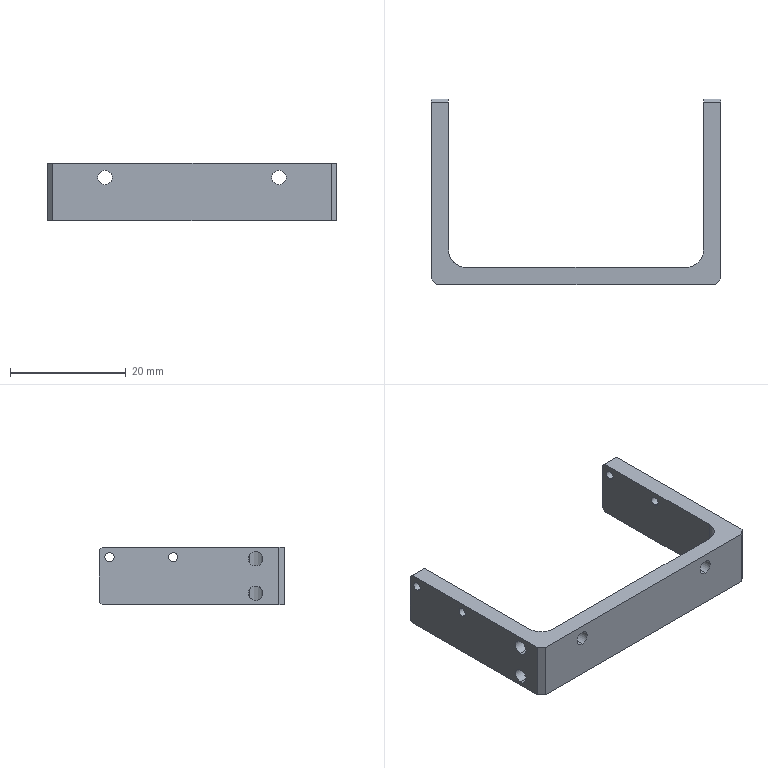Part | SolidWorks | features HoleWzd 3, Chamfer 2, Extrusion 1, Fillet 1, ICE 1 | 1 solid | 34 faces | box 50 x 32 x 10 mm | volume 3182 mm3 | cylinder 18 | plane 16 | commonest cylinder face diameters 1.6 x8 2.5 x8 6 x2
STEP:
#1=CARTESIAN_POINT('',(-21.828,-11.,-4.25));
#2=VERTEX_POINT('',#1);
#3=CARTESIAN_POINT('',(-21.828,-11.,-1.75));
#4=VERTEX_POINT('',#3);
#5=CARTESIAN_POINT('',(-21.828,-11.,-4.25));
#6=CARTESIAN_POINT('',(-21.768,-11.17,-4.25));
#7=CARTESIAN_POINT('',(-21.693,-11.333,-4.215));
#8=CARTESIAN_POINT('',(-21.526,-11.627,-4.093));
#9=CARTESIAN_POINT('',(-21.434,-11.759,-4.005));
#10=CARTESIAN_POINT('',(-21.301,-11.926,-3.843));
#11=CARTESIAN_POINT('',(-21.257,-11.977,-3.784));
#12=CARTESIAN_POINT('',(-21.174,-12.068,-3.654));
#13=CARTESIAN_POINT('',(-21.134,-12.109,-3.583));
#14=CARTESIAN_POINT('',(-21.031,-12.21,-3.356));
#15=CARTESIAN_POINT('',(-20.984,-12.25,-3.178));
#16=CARTESIAN_POINT('',(-20.985,-12.25,-2.817));
#17=CARTESIAN_POINT('',(-21.032,-12.209,-2.642));
#18=CARTESIAN_POINT('',(-21.17,-12.073,-2.338));
#19=CARTESIAN_POINT('',(-21.258,-11.981,-2.209));
#20=CARTESIAN_POINT('',(-21.437,-11.755,-1.992));
#21=CARTESIAN_POINT('',(-21.527,-11.625,-1.906));
#22=CARTESIAN_POINT('',(-21.695,-11.329,-1.784));
#23=CARTESIAN_POINT('',(-21.768,-11.171,-1.75));
#24=CARTESIAN_POINT('',(-21.828,-11.,-1.75));
#25=B_SPLINE_CURVE_WITH_KNOTS('',3,(#5,#6,#7,#8,#9,#10,#11,#12,#13,#14,#15,#16,#17,#18,#19,#20,#21,#22,#23,#24),.UNSPECIFIED.,.F.,.F.,(4,2,2,2,2,2,2,2,2,4),(0.001173,0.001709,0.002246,0.002514,0.002782,0.003319,0.003855,0.004392,0.004928,0.005465),.UNSPECIFIED.);
#26=EDGE_CURVE('',#2,#4,#25,.T.);
#27=ORIENTED_EDGE('',*,*,#26,.F.);
#28=CARTESIAN_POINT('',(-25.,-11.,-4.25));
#29=VERTEX_POINT('',#28);
#30=CARTESIAN_POINT('',(-25.,-11.,-4.25));
#31=DIRECTION('',(-1.,0.,0.));
#32=VECTOR('',#31,1000.);
#33=LINE('',#30,#32);
#34=EDGE_CURVE('',#2,#29,#33,.T.);
#35=ORIENTED_EDGE('',*,*,#34,.T.);
#36=CARTESIAN_POINT('',(-25.,-11.,-1.75));
#37=VERTEX_POINT('',#36);
#38=CARTESIAN_POINT('',(-25.,-11.,-3.));
#39=DIRECTION('',(-1.,0.,0.));
#40=DIRECTION('',(0.,0.,1.));
#41=AXIS2_PLACEMENT_3D('',#38,#39,#40);
#42=CIRCLE('',#41,1.25);
#43=EDGE_CURVE('',#29,#37,#42,.T.);
#44=ORIENTED_EDGE('',*,*,#43,.T.);
#45=CARTESIAN_POINT('',(-25.,-11.,-1.75));
#46=DIRECTION('',(-1.,0.,0.));
#47=VECTOR('',#46,1000.);
#48=LINE('',#45,#47);
#49=EDGE_CURVE('',#4,#37,#48,.T.);
#50=ORIENTED_EDGE('',*,*,#49,.F.);
#51=EDGE_LOOP('',(#27,#35,#44,#50));
#52=FACE_OUTER_BOUND('',#51,.T.);
#53=CARTESIAN_POINT('',(-25.,-11.,-3.));
#54=DIRECTION('',(-1.,0.,0.));
#55=DIRECTION('',(0.,0.,1.));
#56=AXIS2_PLACEMENT_3D('',#53,#54,#55);
#57=CYLINDRICAL_SURFACE('',#56,1.25);
#58=ADVANCED_FACE('',(#52),#57,.F.);
#59=CARTESIAN_POINT('',(-21.828,-11.,1.75));
#60=VERTEX_POINT('',#59);
#61=CARTESIAN_POINT('',(-21.828,-11.,4.25));
#62=VERTEX_POINT('',#61);
#63=CARTESIAN_POINT('',(-21.828,-11.,1.75));
#64=CARTESIAN_POINT('',(-21.768,-11.17,1.75));
#65=CARTESIAN_POINT('',(-21.693,-11.333,1.785));
#66=CARTESIAN_POINT('',(-21.526,-11.627,1.907));
#67=CARTESIAN_POINT('',(-21.434,-11.759,1.995));
#68=CARTESIAN_POINT('',(-21.301,-11.926,2.157));
#69=CARTESIAN_POINT('',(-21.257,-11.977,2.216));
#70=CARTESIAN_POINT('',(-21.174,-12.068,2.346));
#71=CARTESIAN_POINT('',(-21.134,-12.109,2.417));
#72=CARTESIAN_POINT('',(-21.031,-12.21,2.644));
#73=CARTESIAN_POINT('',(-20.984,-12.25,2.822));
#74=CARTESIAN_POINT('',(-20.985,-12.25,3.183));
#75=CARTESIAN_POINT('',(-21.032,-12.209,3.358));
#76=CARTESIAN_POINT('',(-21.17,-12.073,3.662));
#77=CARTESIAN_POINT('',(-21.258,-11.981,3.791));
#78=CARTESIAN_POINT('',(-21.437,-11.755,4.008));
#79=CARTESIAN_POINT('',(-21.527,-11.625,4.094));
#80=CARTESIAN_POINT('',(-21.695,-11.329,4.216));
#81=CARTESIAN_POINT('',(-21.768,-11.171,4.25));
#82=CARTESIAN_POINT('',(-21.828,-11.,4.25));
#83=B_SPLINE_CURVE_WITH_KNOTS('',3,(#63,#64,#65,#66,#67,#68,#69,#70,#71,#72,#73,#74,#75,#76,#77,#78,#79,#80,#81,#82),.UNSPECIFIED.,.F.,.F.,(4,2,2,2,2,2,2,2,2,4),(0.001173,0.001709,0.002246,0.002514,0.002782,0.003319,0.003855,0.004392,0.004928,0.005465),.UNSPECIFIED.);
#84=EDGE_CURVE('',#60,#62,#83,.T.);
#85=ORIENTED_EDGE('',*,*,#84,.F.);
#86=CARTESIAN_POINT('',(-25.,-11.,1.75));
#87=VERTEX_POINT('',#86);
#88=CARTESIAN_POINT('',(-25.,-11.,1.75));
#89=DIRECTION('',(-1.,0.,0.));
#90=VECTOR('',#89,1000.);
#91=LINE('',#88,#90);
#92=EDGE_CURVE('',#60,#87,#91,.T.);
#93=ORIENTED_EDGE('',*,*,#92,.T.);
#94=CARTESIAN_POINT('',(-25.,-11.,4.25));
#95=VERTEX_POINT('',#94);
#96=CARTESIAN_POINT('',(-25.,-11.,3.));
#97=DIRECTION('',(-1.,0.,0.));
#98=DIRECTION('',(0.,0.,1.));
#99=AXIS2_PLACEMENT_3D('',#96,#97,#98);
#100=CIRCLE('',#99,1.25);
#101=EDGE_CURVE('',#87,#95,#100,.T.);
#102=ORIENTED_EDGE('',*,*,#101,.T.);
#103=CARTESIAN_POINT('',(-25.,-11.,4.25));
#104=DIRECTION('',(-1.,0.,0.));
#105=VECTOR('',#104,1000.);
#106=LINE('',#103,#105);
#107=EDGE_CURVE('',#62,#95,#106,.T.);
#108=ORIENTED_EDGE('',*,*,#107,.F.);
#109=EDGE_LOOP('',(#85,#93,#102,#108));
#110=FACE_OUTER_BOUND('',#109,.T.);
#111=CARTESIAN_POINT('',(-25.,-11.,3.));
#112=DIRECTION('',(-1.,0.,0.));
#113=DIRECTION('',(0.,0.,1.));
#114=AXIS2_PLACEMENT_3D('',#111,#112,#113);
#115=CYLINDRICAL_SURFACE('',#114,1.25);
#116=ADVANCED_FACE('',(#110),#115,.F.);
#117=CARTESIAN_POINT('',(-15.,-13.,3.75));
#118=VERTEX_POINT('',#117);
#119=CARTESIAN_POINT('',(-15.,-13.,1.25));
#120=VERTEX_POINT('',#119);
#121=CARTESIAN_POINT('',(-15.,-13.,2.5));
#122=DIRECTION('',(0.,-1.,0.));
#123=DIRECTION('',(0.,0.,-1.));
#124=AXIS2_PLACEMENT_3D('',#121,#122,#123);
#125=CIRCLE('',#124,1.25);
#126=EDGE_CURVE('',#118,#120,#125,.T.);
#127=ORIENTED_EDGE('',*,*,#126,.F.);
#128=CARTESIAN_POINT('',(-15.,-16.,3.75));
#129=VERTEX_POINT('',#128);
#130=CARTESIAN_POINT('',(-15.,-16.,3.75));
#131=DIRECTION('',(0.,-1.,0.));
#132=VECTOR('',#131,1000.);
#133=LINE('',#130,#132);
#134=EDGE_CURVE('',#118,#129,#133,.T.);
#135=ORIENTED_EDGE('',*,*,#134,.T.);
#136=CARTESIAN_POINT('',(-15.,-16.,1.25));
#137=VERTEX_POINT('',#136);
#138=CARTESIAN_POINT('',(-15.,-16.,2.5));
#139=DIRECTION('',(0.,-1.,0.));
#140=DIRECTION('',(0.,0.,-1.));
#141=AXIS2_PLACEMENT_3D('',#138,#139,#140);
#142=CIRCLE('',#141,1.25);
#143=EDGE_CURVE('',#129,#137,#142,.T.);
#144=ORIENTED_EDGE('',*,*,#143,.T.);
#145=CARTESIAN_POINT('',(-15.,-16.,1.25));
#146=DIRECTION('',(0.,-1.,0.));
#147=VECTOR('',#146,1000.);
#148=LINE('',#145,#147);
#149=EDGE_CURVE('',#120,#137,#148,.T.);
#150=ORIENTED_EDGE('',*,*,#149,.F.);
#151=EDGE_LOOP('',(#127,#135,#144,#150));
#152=FACE_OUTER_BOUND('',#151,.T.);
#153=CARTESIAN_POINT('',(-15.,-16.,2.5));
#154=DIRECTION('',(0.,-1.,0.));
#155=DIRECTION('',(0.,0.,-1.));
#156=AXIS2_PLACEMENT_3D('',#153,#154,#155);
#157=CYLINDRICAL_SURFACE('',#156,1.25);
#158=ADVANCED_FACE('',(#152),#157,.F.);
#159=CARTESIAN_POINT('',(15.,-13.,3.75));
#160=VERTEX_POINT('',#159);
#161=CARTESIAN_POINT('',(15.,-13.,1.25));
#162=VERTEX_POINT('',#161);
#163=CARTESIAN_POINT('',(15.,-13.,2.5));
#164=DIRECTION('',(0.,-1.,0.));
#165=DIRECTION('',(0.,0.,-1.));
#166=AXIS2_PLACEMENT_3D('',#163,#164,#165);
#167=CIRCLE('',#166,1.25);
#168=EDGE_CURVE('',#160,#162,#167,.T.);
#169=ORIENTED_EDGE('',*,*,#168,.F.);
#170=CARTESIAN_POINT('',(15.,-16.,3.75));
#171=VERTEX_POINT('',#170);
#172=CARTESIAN_POINT('',(15.,-16.,3.75));
#173=DIRECTION('',(0.,-1.,0.));
#174=VECTOR('',#173,1000.);
#175=LINE('',#172,#174);
#176=EDGE_CURVE('',#160,#171,#175,.T.);
#177=ORIENTED_EDGE('',*,*,#176,.T.);
#178=CARTESIAN_POINT('',(15.,-16.,1.25));
#179=VERTEX_POINT('',#178);
#180=CARTESIAN_POINT('',(15.,-16.,2.5));
#181=DIRECTION('',(0.,-1.,0.));
#182=DIRECTION('',(0.,0.,-1.));
#183=AXIS2_PLACEMENT_3D('',#180,#181,#182);
#184=CIRCLE('',#183,1.25);
#185=EDGE_CURVE('',#171,#179,#184,.T.);
#186=ORIENTED_EDGE('',*,*,#185,.T.);
#187=CARTESIAN_POINT('',(15.,-16.,1.25));
#188=DIRECTION('',(0.,-1.,0.));
#189=VECTOR('',#188,1000.);
#190=LINE('',#187,#189);
#191=EDGE_CURVE('',#162,#179,#190,.T.);
#192=ORIENTED_EDGE('',*,*,#191,.F.);
#193=EDGE_LOOP('',(#169,#177,#186,#192));
#194=FACE_OUTER_BOUND('',#193,.T.);
#195=CARTESIAN_POINT('',(15.,-16.,2.5));
#196=DIRECTION('',(0.,-1.,0.));
#197=DIRECTION('',(0.,0.,-1.));
#198=AXIS2_PLACEMENT_3D('',#195,#196,#197);
#199=CYLINDRICAL_SURFACE('',#198,1.25);
#200=ADVANCED_FACE('',(#194),#199,.F.);
#201=CARTESIAN_POINT('',(22.,14.25,4.05));
#202=VERTEX_POINT('',#201);
#203=CARTESIAN_POINT('',(22.,14.25,2.45));
#204=VERTEX_POINT('',#203);
#205=CARTESIAN_POINT('',(22.,14.25,3.25));
#206=DIRECTION('',(1.,0.,0.));
#207=DIRECTION('',(0.,0.,-1.));
#208=AXIS2_PLACEMENT_3D('',#205,#206,#207);
#209=CIRCLE('',#208,0.8);
#210=EDGE_CURVE('',#202,#204,#209,.T.);
#211=ORIENTED_EDGE('',*,*,#210,.F.);
#212=CARTESIAN_POINT('',(25.,14.25,4.05));
#213=VERTEX_POINT('',#212);
#214=CARTESIAN_POINT('',(25.,14.25,4.05));
#215=DIRECTION('',(1.,0.,0.));
#216=VECTOR('',#215,1000.);
#217=LINE('',#214,#216);
#218=EDGE_CURVE('',#202,#213,#217,.T.);
#219=ORIENTED_EDGE('',*,*,#218,.T.);
#220=CARTESIAN_POINT('',(25.,14.25,2.45));
#221=VERTEX_POINT('',#220);
#222=CARTESIAN_POINT('',(25.,14.25,3.25));
#223=DIRECTION('',(1.,0.,0.));
#224=DIRECTION('',(0.,0.,-1.));
#225=AXIS2_PLACEMENT_3D('',#222,#223,#224);
#226=CIRCLE('',#225,0.8);
#227=EDGE_CURVE('',#213,#221,#226,.T.);
#228=ORIENTED_EDGE('',*,*,#227,.T.);
#229=CARTESIAN_POINT('',(25.,14.25,2.45));
#230=DIRECTION('',(1.,0.,0.));
#231=VECTOR('',#230,1000.);
#232=LINE('',#229,#231);
#233=EDGE_CURVE('',#204,#221,#232,.T.);
#234=ORIENTED_EDGE('',*,*,#233,.F.);
#235=EDGE_LOOP('',(#211,#219,#228,#234));
#236=FACE_OUTER_BOUND('',#235,.T.);
#237=CARTESIAN_POINT('',(25.,14.25,3.25));
#238=DIRECTION('',(1.,0.,0.));
#239=DIRECTION('',(0.,0.,-1.));
#240=AXIS2_PLACEMENT_3D('',#237,#238,#239);
#241=CYLINDRICAL_SURFACE('',#240,0.8);
#242=ADVANCED_FACE('',(#236),#241,.F.);
#243=CARTESIAN_POINT('',(-25.,14.25,4.05));
#244=VERTEX_POINT('',#243);
#245=CARTESIAN_POINT('',(-25.,14.25,2.45));
#246=VERTEX_POINT('',#245);
#247=CARTESIAN_POINT('',(-25.,14.25,3.25));
#248=DIRECTION('',(1.,0.,0.));
#249=DIRECTION('',(0.,0.,-1.));
#250=AXIS2_PLACEMENT_3D('',#247,#248,#249);
#251=CIRCLE('',#250,0.8);
#252=EDGE_CURVE('',#244,#246,#251,.T.);
#253=ORIENTED_EDGE('',*,*,#252,.F.);
#254=CARTESIAN_POINT('',(-22.,14.25,4.05));
#255=VERTEX_POINT('',#254);
#256=CARTESIAN_POINT('',(25.,14.25,4.05));
#257=DIRECTION('',(1.,0.,0.));
#258=VECTOR('',#257,1000.);
#259=LINE('',#256,#258);
#260=EDGE_CURVE('',#244,#255,#259,.T.);
#261=ORIENTED_EDGE('',*,*,#260,.T.);
#262=CARTESIAN_POINT('',(-22.,14.25,2.45));
#263=VERTEX_POINT('',#262);
#264=CARTESIAN_POINT('',(-22.,14.25,3.25));
#265=DIRECTION('',(-1.,0.,0.));
#266=DIRECTION('',(0.,0.,1.));
#267=AXIS2_PLACEMENT_3D('',#264,#265,#266);
#268=CIRCLE('',#267,0.8);
#269=EDGE_CURVE('',#263,#255,#268,.T.);
#270=ORIENTED_EDGE('',*,*,#269,.F.);
#271=CARTESIAN_POINT('',(25.,14.25,2.45));
#272=DIRECTION('',(1.,0.,0.));
#273=VECTOR('',#272,1000.);
#274=LINE('',#271,#273);
#275=EDGE_CURVE('',#246,#263,#274,.T.);
#276=ORIENTED_EDGE('',*,*,#275,.F.);
#277=EDGE_LOOP('',(#253,#261,#270,#276));
#278=FACE_OUTER_BOUND('',#277,.T.);
#279=CARTESIAN_POINT('',(25.,14.25,3.25));
#280=DIRECTION('',(1.,0.,0.));
#281=DIRECTION('',(0.,0.,-1.));
#282=AXIS2_PLACEMENT_3D('',#279,#280,#281);
#283=CYLINDRICAL_SURFACE('',#282,0.8);
#284=ADVANCED_FACE('',(#278),#283,.F.);
#285=CARTESIAN_POINT('',(22.,3.25,4.05));
#286=VERTEX_POINT('',#285);
#287=CARTESIAN_POINT('',(22.,3.25,2.45));
#288=VERTEX_POINT('',#287);
#289=CARTESIAN_POINT('',(22.,3.25,3.25));
#290=DIRECTION('',(1.,0.,0.));
#291=DIRECTION('',(0.,0.,-1.));
#292=AXIS2_PLACEMENT_3D('',#289,#290,#291);
#293=CIRCLE('',#292,0.8);
#294=EDGE_CURVE('',#286,#288,#293,.T.);
#295=ORIENTED_EDGE('',*,*,#294,.F.);
#296=CARTESIAN_POINT('',(25.,3.25,4.05));
#297=VERTEX_POINT('',#296);
#298=CARTESIAN_POINT('',(25.,3.25,4.05));
#299=DIRECTION('',(1.,0.,0.));
#300=VECTOR('',#299,1000.);
#301=LINE('',#298,#300);
#302=EDGE_CURVE('',#286,#297,#301,.T.);
#303=ORIENTED_EDGE('',*,*,#302,.T.);
#304=CARTESIAN_POINT('',(25.,3.25,2.45));
#305=VERTEX_POINT('',#304);
#306=CARTESIAN_POINT('',(25.,3.25,3.25));
#307=DIRECTION('',(1.,0.,0.));
#308=DIRECTION('',(0.,0.,-1.));
#309=AXIS2_PLACEMENT_3D('',#306,#307,#308);
#310=CIRCLE('',#309,0.8);
#311=EDGE_CURVE('',#297,#305,#310,.T.);
#312=ORIENTED_EDGE('',*,*,#311,.T.);
#313=CARTESIAN_POINT('',(25.,3.25,2.45));
#314=DIRECTION('',(1.,0.,0.));
#315=VECTOR('',#314,1000.);
#316=LINE('',#313,#315);
#317=EDGE_CURVE('',#288,#305,#316,.T.);
#318=ORIENTED_EDGE('',*,*,#317,.F.);
#319=EDGE_LOOP('',(#295,#303,#312,#318));
#320=FACE_OUTER_BOUND('',#319,.T.);
#321=CARTESIAN_POINT('',(25.,3.25,3.25));
#322=DIRECTION('',(1.,0.,0.));
#323=DIRECTION('',(0.,0.,-1.));
#324=AXIS2_PLACEMENT_3D('',#321,#322,#323);
#325=CYLINDRICAL_SURFACE('',#324,0.8);
#326=ADVANCED_FACE('',(#320),#325,.F.);
#327=CARTESIAN_POINT('',(-25.,3.25,4.05));
#328=VERTEX_POINT('',#327);
#329=CARTESIAN_POINT('',(-25.,3.25,2.45));
#330=VERTEX_POINT('',#329);
#331=CARTESIAN_POINT('',(-25.,3.25,3.25));
#332=DIRECTION('',(1.,0.,0.));
#333=DIRECTION('',(0.,0.,-1.));
#334=AXIS2_PLACEMENT_3D('',#331,#332,#333);
#335=CIRCLE('',#334,0.8);
#336=EDGE_CURVE('',#328,#330,#335,.T.);
#337=ORIENTED_EDGE('',*,*,#336,.F.);
#338=CARTESIAN_POINT('',(-22.,3.25,4.05));
#339=VERTEX_POINT('',#338);
#340=CARTESIAN_POINT('',(25.,3.25,4.05));
#341=DIRECTION('',(1.,0.,0.));
#342=VECTOR('',#341,1000.);
#343=LINE('',#340,#342);
#344=EDGE_CURVE('',#328,#339,#343,.T.);
#345=ORIENTED_EDGE('',*,*,#344,.T.);
#346=CARTESIAN_POINT('',(-22.,3.25,2.45));
#347=VERTEX_POINT('',#346);
#348=CARTESIAN_POINT('',(-22.,3.25,3.25));
#349=DIRECTION('',(-1.,0.,0.));
#350=DIRECTION('',(0.,0.,1.));
#351=AXIS2_PLACEMENT_3D('',#348,#349,#350);
#352=CIRCLE('',#351,0.8);
#353=EDGE_CURVE('',#347,#339,#352,.T.);
#354=ORIENTED_EDGE('',*,*,#353,.F.);
#355=CARTESIAN_POINT('',(25.,3.25,2.45));
#356=DIRECTION('',(1.,0.,0.));
#357=VECTOR('',#356,1000.);
#358=LINE('',#355,#357);
#359=EDGE_CURVE('',#330,#347,#358,.T.);
#360=ORIENTED_EDGE('',*,*,#359,.F.);
#361=EDGE_LOOP('',(#337,#345,#354,#360));
#362=FACE_OUTER_BOUND('',#361,.T.);
#363=CARTESIAN_POINT('',(25.,3.25,3.25));
#364=DIRECTION('',(1.,0.,0.));
#365=DIRECTION('',(0.,0.,-1.));
#366=AXIS2_PLACEMENT_3D('',#363,#364,#365);
#367=CYLINDRICAL_SURFACE('',#366,0.8);
#368=ADVANCED_FACE('',(#362),#367,.F.);
#369=CARTESIAN_POINT('',(22.,16.,-4.5));
#370=VERTEX_POINT('',#369);
#371=CARTESIAN_POINT('',(22.,16.,4.5));
#372=VERTEX_POINT('',#371);
#373=CARTESIAN_POINT('',(22.,16.,-5.));
#374=DIRECTION('',(0.,0.,1.));
#375=VECTOR('',#374,1000.);
#376=LINE('',#373,#375);
#377=EDGE_CURVE('',#370,#372,#376,.T.);
#378=ORIENTED_EDGE('',*,*,#377,.T.);
#379=CARTESIAN_POINT('',(25.,16.,4.5));
#380=VERTEX_POINT('',#379);
#381=CARTESIAN_POINT('',(25.,16.,4.5));
#382=DIRECTION('',(1.,0.,0.));
#383=VECTOR('',#382,1000.);
#384=LINE('',#381,#383);
#385=EDGE_CURVE('',#372,#380,#384,.T.);
#386=ORIENTED_EDGE('',*,*,#385,.T.);
#387=CARTESIAN_POINT('',(25.,16.,-4.5));
#388=VERTEX_POINT('',#387);
#389=CARTESIAN_POINT('',(25.,16.,5.));
#390=DIRECTION('',(0.,0.,-1.));
#391=VECTOR('',#390,1000.);
#392=LINE('',#389,#391);
#393=EDGE_CURVE('',#380,#388,#392,.T.);
#394=ORIENTED_EDGE('',*,*,#393,.T.);
#395=CARTESIAN_POINT('',(-25.,16.,-4.5));
#396=DIRECTION('',(-1.,0.,0.));
#397=VECTOR('',#396,1000.);
#398=LINE('',#395,#397);
#399=EDGE_CURVE('',#388,#370,#398,.T.);
#400=ORIENTED_EDGE('',*,*,#399,.T.);
#401=EDGE_LOOP('',(#378,#386,#394,#400));
#402=FACE_OUTER_BOUND('',#401,.T.);
#403=CARTESIAN_POINT('',(-25.,16.,5.));
#404=DIRECTION('',(0.,-1.,0.));
#405=DIRECTION('',(0.,0.,-1.));
#406=AXIS2_PLACEMENT_3D('',#403,#404,#405);
#407=PLANE('',#406);
#408=ADVANCED_FACE('',(#402),#407,.F.);
#409=CARTESIAN_POINT('',(25.,14.25,3.25));
#410=DIRECTION('',(1.,0.,0.));
#411=DIRECTION('',(0.,0.,-1.));
#412=AXIS2_PLACEMENT_3D('',#409,#410,#411);
#413=CIRCLE('',#412,0.8);
#414=EDGE_CURVE('',#221,#213,#413,.T.);
#415=ORIENTED_EDGE('',*,*,#414,.F.);
#416=ORIENTED_EDGE('',*,*,#227,.F.);
#417=EDGE_LOOP('',(#415,#416));
#418=FACE_BOUND('',#417,.T.);
#419=CARTESIAN_POINT('',(25.,3.25,3.25));
#420=DIRECTION('',(1.,0.,0.));
#421=DIRECTION('',(0.,0.,-1.));
#422=AXIS2_PLACEMENT_3D('',#419,#420,#421);
#423=CIRCLE('',#422,0.8);
#424=EDGE_CURVE('',#305,#297,#423,.T.);
#425=ORIENTED_EDGE('',*,*,#424,.F.);
#426=ORIENTED_EDGE('',*,*,#311,.F.);
#427=EDGE_LOOP('',(#425,#426));
#428=FACE_BOUND('',#427,.T.);
#429=CARTESIAN_POINT('',(25.,-15.,5.));
#430=VERTEX_POINT('',#429);
#431=CARTESIAN_POINT('',(25.,15.5,5.));
#432=VERTEX_POINT('',#431);
#433=CARTESIAN_POINT('',(25.,16.,5.));
#434=DIRECTION('',(0.,1.,0.));
#435=VECTOR('',#434,1000.);
#436=LINE('',#433,#435);
#437=EDGE_CURVE('',#430,#432,#436,.T.);
#438=ORIENTED_EDGE('',*,*,#437,.F.);
#439=CARTESIAN_POINT('',(25.,-15.,-5.));
#440=VERTEX_POINT('',#439);
#441=CARTESIAN_POINT('',(25.,-15.,5.));
#442=DIRECTION('',(0.,0.,-1.));
#443=VECTOR('',#442,1000.);
#444=LINE('',#441,#443);
#445=EDGE_CURVE('',#430,#440,#444,.T.);
#446=ORIENTED_EDGE('',*,*,#445,.T.);
#447=CARTESIAN_POINT('',(25.,15.5,-5.));
#448=VERTEX_POINT('',#447);
#449=CARTESIAN_POINT('',(25.,16.,-5.));
#450=DIRECTION('',(0.,1.,0.));
#451=VECTOR('',#450,1000.);
#452=LINE('',#449,#451);
#453=EDGE_CURVE('',#440,#448,#452,.T.);
#454=ORIENTED_EDGE('',*,*,#453,.T.);
#455=CARTESIAN_POINT('',(25.,16.,-4.5));
#456=DIRECTION('',(0.,0.7071,0.7071));
#457=VECTOR('',#456,1000.);
#458=LINE('',#455,#457);
#459=EDGE_CURVE('',#448,#388,#458,.T.);
#460=ORIENTED_EDGE('',*,*,#459,.T.);
#461=ORIENTED_EDGE('',*,*,#393,.F.);
#462=CARTESIAN_POINT('',(25.,15.5,5.));
#463=DIRECTION('',(0.,-0.7071,0.7071));
#464=VECTOR('',#463,1000.);
#465=LINE('',#462,#464);
#466=EDGE_CURVE('',#380,#432,#465,.T.);
#467=ORIENTED_EDGE('',*,*,#466,.T.);
#468=EDGE_LOOP('',(#438,#446,#454,#460,#461,#467));
#469=FACE_OUTER_BOUND('',#468,.T.);
#470=CARTESIAN_POINT('',(25.,16.,5.));
#471=DIRECTION('',(-1.,0.,0.));
#472=DIRECTION('',(0.,-1.,0.));
#473=AXIS2_PLACEMENT_3D('',#470,#471,#472);
#474=PLANE('',#473);
#475=ADVANCED_FACE('',(#418,#428,#469),#474,.F.);
#476=CARTESIAN_POINT('',(-22.,16.,-4.5));
#477=VERTEX_POINT('',#476);
#478=CARTESIAN_POINT('',(-22.,16.,4.5));
#479=VERTEX_POINT('',#478);
#480=CARTESIAN_POINT('',(-22.,16.,-5.));
#481=DIRECTION('',(0.,0.,1.));
#482=VECTOR('',#481,1000.);
#483=LINE('',#480,#482);
#484=EDGE_CURVE('',#477,#479,#483,.T.);
#485=ORIENTED_EDGE('',*,*,#484,.F.);
#486=CARTESIAN_POINT('',(-25.,16.,-4.5));
#487=VERTEX_POINT('',#486);
#488=CARTESIAN_POINT('',(-25.,16.,-4.5));
#489=DIRECTION('',(-1.,0.,0.));
#490=VECTOR('',#489,1000.);
#491=LINE('',#488,#490);
#492=EDGE_CURVE('',#477,#487,#491,.T.);
#493=ORIENTED_EDGE('',*,*,#492,.T.);
#494=CARTESIAN_POINT('',(-25.,16.,4.5));
#495=VERTEX_POINT('',#494);
#496=CARTESIAN_POINT('',(-25.,16.,5.));
#497=DIRECTION('',(0.,0.,-1.));
#498=VECTOR('',#497,1000.);
#499=LINE('',#496,#498);
#500=EDGE_CURVE('',#495,#487,#499,.T.);
#501=ORIENTED_EDGE('',*,*,#500,.F.);
#502=CARTESIAN_POINT('',(-22.,16.,4.5));
#503=DIRECTION('',(1.,0.,0.));
#504=VECTOR('',#503,1000.);
#505=LINE('',#502,#504);
#506=EDGE_CURVE('',#495,#479,#505,.T.);
#507=ORIENTED_EDGE('',*,*,#506,.T.);
#508=EDGE_LOOP('',(#485,#493,#501,#507));
#509=FACE_OUTER_BOUND('',#508,.T.);
#510=CARTESIAN_POINT('',(-25.,16.,5.));
#511=DIRECTION('',(0.,-1.,0.));
#512=DIRECTION('',(0.,0.,-1.));
#513=AXIS2_PLACEMENT_3D('',#510,#511,#512);
#514=PLANE('',#513);
#515=ADVANCED_FACE('',(#509),#514,.F.);
#516=CARTESIAN_POINT('',(-25.,-11.,-3.));
#517=DIRECTION('',(-1.,0.,0.));
#518=DIRECTION('',(0.,0.,1.));
#519=AXIS2_PLACEMENT_3D('',#516,#517,#518);
#520=CIRCLE('',#519,1.25);
#521=EDGE_CURVE('',#37,#29,#520,.T.);
#522=ORIENTED_EDGE('',*,*,#521,.F.);
#523=ORIENTED_EDGE('',*,*,#43,.F.);
#524=EDGE_LOOP('',(#522,#523));
#525=FACE_BOUND('',#524,.T.);
#526=CARTESIAN_POINT('',(-25.,-11.,3.));
#527=DIRECTION('',(-1.,0.,0.));
#528=DIRECTION('',(0.,0.,1.));
#529=AXIS2_PLACEMENT_3D('',#526,#527,#528);
#530=CIRCLE('',#529,1.25);
#531=EDGE_CURVE('',#95,#87,#530,.T.);
#532=ORIENTED_EDGE('',*,*,#531,.F.);
#533=ORIENTED_EDGE('',*,*,#101,.F.);
#534=EDGE_LOOP('',(#532,#533));
#535=FACE_BOUND('',#534,.T.);
#536=CARTESIAN_POINT('',(-25.,14.25,3.25));
#537=DIRECTION('',(1.,0.,0.));
#538=DIRECTION('',(0.,0.,-1.));
#539=AXIS2_PLACEMENT_3D('',#536,#537,#538);
#540=CIRCLE('',#539,0.8);
#541=EDGE_CURVE('',#246,#244,#540,.T.);
#542=ORIENTED_EDGE('',*,*,#541,.T.);
#543=ORIENTED_EDGE('',*,*,#252,.T.);
#544=EDGE_LOOP('',(#542,#543));
#545=FACE_BOUND('',#544,.T.);
#546=CARTESIAN_POINT('',(-25.,3.25,3.25));
#547=DIRECTION('',(1.,0.,0.));
#548=DIRECTION('',(0.,0.,-1.));
#549=AXIS2_PLACEMENT_3D('',#546,#547,#548);
#550=CIRCLE('',#549,0.8);
#551=EDGE_CURVE('',#330,#328,#550,.T.);
#552=ORIENTED_EDGE('',*,*,#551,.T.);
#553=ORIENTED_EDGE('',*,*,#336,.T.);
#554=EDGE_LOOP('',(#552,#553));
#555=FACE_BOUND('',#554,.T.);
#556=CARTESIAN_POINT('',(-25.,15.5,-5.));
#557=VERTEX_POINT('',#556);
#558=CARTESIAN_POINT('',(-25.,-15.,-5.));
#559=VERTEX_POINT('',#558);
#560=CARTESIAN_POINT('',(-25.,16.,-5.));
#561=DIRECTION('',(0.,-1.,0.));
#562=VECTOR('',#561,1000.);
#563=LINE('',#560,#562);
#564=EDGE_CURVE('',#557,#559,#563,.T.);
#565=ORIENTED_EDGE('',*,*,#564,.T.);
#566=CARTESIAN_POINT('',(-25.,-15.,5.));
#567=VERTEX_POINT('',#566);
#568=CARTESIAN_POINT('',(-25.,-15.,5.));
#569=DIRECTION('',(0.,0.,1.));
#570=VECTOR('',#569,1000.);
#571=LINE('',#568,#570);
#572=EDGE_CURVE('',#559,#567,#571,.T.);
#573=ORIENTED_EDGE('',*,*,#572,.T.);
#574=CARTESIAN_POINT('',(-25.,15.5,5.));
#575=VERTEX_POINT('',#574);
#576=CARTESIAN_POINT('',(-25.,16.,5.));
#577=DIRECTION('',(0.,-1.,0.));
#578=VECTOR('',#577,1000.);
#579=LINE('',#576,#578);
#580=EDGE_CURVE('',#575,#567,#579,.T.);
#581=ORIENTED_EDGE('',*,*,#580,.F.);
#582=CARTESIAN_POINT('',(-25.,15.5,5.));
#583=DIRECTION('',(0.,0.7071,-0.7071));
#584=VECTOR('',#583,1000.);
#585=LINE('',#582,#584);
#586=EDGE_CURVE('',#575,#495,#585,.T.);
#587=ORIENTED_EDGE('',*,*,#586,.T.);
#588=ORIENTED_EDGE('',*,*,#500,.T.);
#589=CARTESIAN_POINT('',(-25.,16.,-4.5));
#590=DIRECTION('',(0.,-0.7071,-0.7071));
#591=VECTOR('',#590,1000.);
#592=LINE('',#589,#591);
#593=EDGE_CURVE('',#487,#557,#592,.T.);
#594=ORIENTED_EDGE('',*,*,#593,.T.);
#595=EDGE_LOOP('',(#565,#573,#581,#587,#588,#594));
#596=FACE_OUTER_BOUND('',#595,.T.);
#597=CARTESIAN_POINT('',(-25.,16.,5.));
#598=DIRECTION('',(1.,0.,0.));
#599=DIRECTION('',(0.,1.,0.));
#600=AXIS2_PLACEMENT_3D('',#597,#598,#599);
#601=PLANE('',#600);
#602=ADVANCED_FACE('',(#525,#535,#545,#555,#596),#601,.F.);
#603=CARTESIAN_POINT('',(-15.,-16.,2.5));
#604=DIRECTION('',(0.,-1.,0.));
#605=DIRECTION('',(0.,0.,-1.));
#606=AXIS2_PLACEMENT_3D('',#603,#604,#605);
#607=CIRCLE('',#606,1.25);
#608=EDGE_CURVE('',#137,#129,#607,.T.);
#609=ORIENTED_EDGE('',*,*,#608,.F.);
#610=ORIENTED_EDGE('',*,*,#143,.F.);
#611=EDGE_LOOP('',(#609,#610));
#612=FACE_BOUND('',#611,.T.);
#613=CARTESIAN_POINT('',(15.,-16.,2.5));
#614=DIRECTION('',(0.,-1.,0.));
#615=DIRECTION('',(0.,0.,-1.));
#616=AXIS2_PLACEMENT_3D('',#613,#614,#615);
#617=CIRCLE('',#616,1.25);
#618=EDGE_CURVE('',#179,#171,#617,.T.);
#619=ORIENTED_EDGE('',*,*,#618,.F.);
#620=ORIENTED_EDGE('',*,*,#185,.F.);
#621=EDGE_LOOP('',(#619,#620));
#622=FACE_BOUND('',#621,.T.);
#623=CARTESIAN_POINT('',(-24.,-16.,5.));
#624=VERTEX_POINT('',#623);
#625=CARTESIAN_POINT('',(24.,-16.,5.));
#626=VERTEX_POINT('',#625);
#627=CARTESIAN_POINT('',(-25.,-16.,5.));
#628=DIRECTION('',(1.,0.,0.));
#629=VECTOR('',#628,1000.);
#630=LINE('',#627,#629);
#631=EDGE_CURVE('',#624,#626,#630,.T.);
#632=ORIENTED_EDGE('',*,*,#631,.F.);
#633=CARTESIAN_POINT('',(-24.,-16.,-5.));
#634=VERTEX_POINT('',#633);
#635=CARTESIAN_POINT('',(-24.,-16.,5.));
#636=DIRECTION('',(0.,0.,-1.));
#637=VECTOR('',#636,1000.);
#638=LINE('',#635,#637);
#639=EDGE_CURVE('',#624,#634,#638,.T.);
#640=ORIENTED_EDGE('',*,*,#639,.T.);
#641=CARTESIAN_POINT('',(24.,-16.,-5.));
#642=VERTEX_POINT('',#641);
#643=CARTESIAN_POINT('',(-25.,-16.,-5.));
#644=DIRECTION('',(1.,0.,0.));
#645=VECTOR('',#644,1000.);
#646=LINE('',#643,#645);
#647=EDGE_CURVE('',#634,#642,#646,.T.);
#648=ORIENTED_EDGE('',*,*,#647,.T.);
#649=CARTESIAN_POINT('',(24.,-16.,5.));
#650=DIRECTION('',(0.,0.,1.));
#651=VECTOR('',#650,1000.);
#652=LINE('',#649,#651);
#653=EDGE_CURVE('',#642,#626,#652,.T.);
#654=ORIENTED_EDGE('',*,*,#653,.T.);
#655=EDGE_LOOP('',(#632,#640,#648,#654));
#656=FACE_OUTER_BOUND('',#655,.T.);
#657=CARTESIAN_POINT('',(-25.,-16.,5.));
#658=DIRECTION('',(0.,1.,0.));
#659=DIRECTION('',(0.,0.,1.));
#660=AXIS2_PLACEMENT_3D('',#657,#658,#659);
#661=PLANE('',#660);
#662=ADVANCED_FACE('',(#612,#622,#656),#661,.F.);
#663=ORIENTED_EDGE('',*,*,#580,.T.);
#664=CARTESIAN_POINT('',(-20.,-20.,5.));
#665=DIRECTION('',(0.7071,-0.7071,0.));
#666=VECTOR('',#665,1000.);
#667=LINE('',#664,#666);
#668=EDGE_CURVE('',#567,#624,#667,.T.);
#669=ORIENTED_EDGE('',*,*,#668,.T.);
#670=ORIENTED_EDGE('',*,*,#631,.T.);
#671=CARTESIAN_POINT('',(20.,-20.,5.));
#672=DIRECTION('',(0.7071,0.7071,0.));
#673=VECTOR('',#672,1000.);
#674=LINE('',#671,#673);
#675=EDGE_CURVE('',#626,#430,#674,.T.);
#676=ORIENTED_EDGE('',*,*,#675,.T.);
#677=ORIENTED_EDGE('',*,*,#437,.T.);
#678=CARTESIAN_POINT('',(22.,15.5,5.));
#679=VERTEX_POINT('',#678);
#680=CARTESIAN_POINT('',(22.,15.5,5.));
#681=DIRECTION('',(-1.,0.,0.));
#682=VECTOR('',#681,1000.);
#683=LINE('',#680,#682);
#684=EDGE_CURVE('',#432,#679,#683,.T.);
#685=ORIENTED_EDGE('',*,*,#684,.T.);
#686=CARTESIAN_POINT('',(22.,-10.,5.));
#687=VERTEX_POINT('',#686);
#688=CARTESIAN_POINT('',(22.,16.,5.));
#689=DIRECTION('',(0.,1.,0.));
#690=VECTOR('',#689,1000.);
#691=LINE('',#688,#690);
#692=EDGE_CURVE('',#687,#679,#691,.T.);
#693=ORIENTED_EDGE('',*,*,#692,.F.);
#694=CARTESIAN_POINT('',(19.,-13.,5.));
#695=VERTEX_POINT('',#694);
#696=CARTESIAN_POINT('',(19.,-10.,5.));
#697=DIRECTION('',(0.,0.,-1.));
#698=DIRECTION('',(1.,0.,0.));
#699=AXIS2_PLACEMENT_3D('',#696,#697,#698);
#700=CIRCLE('',#699,3.);
#701=EDGE_CURVE('',#687,#695,#700,.T.);
#702=ORIENTED_EDGE('',*,*,#701,.T.);
#703=CARTESIAN_POINT('',(-19.,-13.,5.));
#704=VERTEX_POINT('',#703);
#705=CARTESIAN_POINT('',(-22.,-13.,5.));
#706=DIRECTION('',(1.,0.,0.));
#707=VECTOR('',#706,1000.);
#708=LINE('',#705,#707);
#709=EDGE_CURVE('',#704,#695,#708,.T.);
#710=ORIENTED_EDGE('',*,*,#709,.F.);
#711=CARTESIAN_POINT('',(-22.,-10.,5.));
#712=VERTEX_POINT('',#711);
#713=CARTESIAN_POINT('',(-19.,-10.,5.));
#714=DIRECTION('',(0.,0.,-1.));
#715=DIRECTION('',(1.,0.,0.));
#716=AXIS2_PLACEMENT_3D('',#713,#714,#715);
#717=CIRCLE('',#716,3.);
#718=EDGE_CURVE('',#704,#712,#717,.T.);
#719=ORIENTED_EDGE('',*,*,#718,.T.);
#720=CARTESIAN_POINT('',(-22.,15.5,5.));
#721=VERTEX_POINT('',#720);
#722=CARTESIAN_POINT('',(-22.,16.,5.));
#723=DIRECTION('',(0.,-1.,0.));
#724=VECTOR('',#723,1000.);
#725=LINE('',#722,#724);
#726=EDGE_CURVE('',#721,#712,#725,.T.);
#727=ORIENTED_EDGE('',*,*,#726,.F.);
#728=CARTESIAN_POINT('',(-25.,15.5,5.));
#729=DIRECTION('',(-1.,0.,0.));
#730=VECTOR('',#729,1000.);
#731=LINE('',#728,#730);
#732=EDGE_CURVE('',#721,#575,#731,.T.);
#733=ORIENTED_EDGE('',*,*,#732,.T.);
#734=EDGE_LOOP('',(#663,#669,#670,#676,#677,#685,#693,#702,#710,#719,#727,#733));
#735=FACE_OUTER_BOUND('',#734,.T.);
#736=CARTESIAN_POINT('',(0.,0.,5.));
#737=DIRECTION('',(0.,0.,1.));
#738=DIRECTION('',(1.,0.,0.));
#739=AXIS2_PLACEMENT_3D('',#736,#737,#738);
#740=PLANE('',#739);
#741=ADVANCED_FACE('',(#735),#740,.T.);
#742=ORIENTED_EDGE('',*,*,#647,.F.);
#743=CARTESIAN_POINT('',(-24.,-16.,-5.));
#744=DIRECTION('',(-0.7071,0.7071,0.));
#745=VECTOR('',#744,1000.);
#746=LINE('',#743,#745);
#747=EDGE_CURVE('',#634,#559,#746,.T.);
#748=ORIENTED_EDGE('',*,*,#747,.T.);
#749=ORIENTED_EDGE('',*,*,#564,.F.);
#750=CARTESIAN_POINT('',(-22.,15.5,-5.));
#751=VERTEX_POINT('',#750);
#752=CARTESIAN_POINT('',(0.,15.5,-5.));
#753=DIRECTION('',(1.,0.,0.));
#754=VECTOR('',#753,1000.);
#755=LINE('',#752,#754);
#756=EDGE_CURVE('',#557,#751,#755,.T.);
#757=ORIENTED_EDGE('',*,*,#756,.T.);
#758=CARTESIAN_POINT('',(-22.,-10.,-5.));
#759=VERTEX_POINT('',#758);
#760=CARTESIAN_POINT('',(-22.,16.,-5.));
#761=DIRECTION('',(0.,-1.,0.));
#762=VECTOR('',#761,1000.);
#763=LINE('',#760,#762);
#764=EDGE_CURVE('',#751,#759,#763,.T.);
#765=ORIENTED_EDGE('',*,*,#764,.T.);
#766=CARTESIAN_POINT('',(-19.,-13.,-5.));
#767=VERTEX_POINT('',#766);
#768=CARTESIAN_POINT('',(-19.,-10.,-5.));
#769=DIRECTION('',(0.,0.,1.));
#770=DIRECTION('',(1.,0.,0.));
#771=AXIS2_PLACEMENT_3D('',#768,#769,#770);
#772=CIRCLE('',#771,3.);
#773=EDGE_CURVE('',#759,#767,#772,.T.);
#774=ORIENTED_EDGE('',*,*,#773,.T.);
#775=CARTESIAN_POINT('',(19.,-13.,-5.));
#776=VERTEX_POINT('',#775);
#777=CARTESIAN_POINT('',(-22.,-13.,-5.));
#778=DIRECTION('',(1.,0.,0.));
#779=VECTOR('',#778,1000.);
#780=LINE('',#777,#779);
#781=EDGE_CURVE('',#767,#776,#780,.T.);
#782=ORIENTED_EDGE('',*,*,#781,.T.);
#783=CARTESIAN_POINT('',(22.,-10.,-5.));
#784=VERTEX_POINT('',#783);
#785=CARTESIAN_POINT('',(19.,-10.,-5.));
#786=DIRECTION('',(0.,0.,1.));
#787=DIRECTION('',(1.,0.,0.));
#788=AXIS2_PLACEMENT_3D('',#785,#786,#787);
#789=CIRCLE('',#788,3.);
#790=EDGE_CURVE('',#776,#784,#789,.T.);
#791=ORIENTED_EDGE('',*,*,#790,.T.);
#792=CARTESIAN_POINT('',(22.,15.5,-5.));
#793=VERTEX_POINT('',#792);
#794=CARTESIAN_POINT('',(22.,16.,-5.));
#795=DIRECTION('',(0.,1.,0.));
#796=VECTOR('',#795,1000.);
#797=LINE('',#794,#796);
#798=EDGE_CURVE('',#784,#793,#797,.T.);
#799=ORIENTED_EDGE('',*,*,#798,.T.);
#800=CARTESIAN_POINT('',(0.,15.5,-5.));
#801=DIRECTION('',(1.,0.,0.));
#802=VECTOR('',#801,1000.);
#803=LINE('',#800,#802);
#804=EDGE_CURVE('',#793,#448,#803,.T.);
#805=ORIENTED_EDGE('',*,*,#804,.T.);
#806=ORIENTED_EDGE('',*,*,#453,.F.);
#807=CARTESIAN_POINT('',(25.,-15.,-5.));
#808=DIRECTION('',(-0.7071,-0.7071,0.));
#809=VECTOR('',#808,1000.);
#810=LINE('',#807,#809);
#811=EDGE_CURVE('',#440,#642,#810,.T.);
#812=ORIENTED_EDGE('',*,*,#811,.T.);
#813=EDGE_LOOP('',(#742,#748,#749,#757,#765,#774,#782,#791,#799,#805,#806,#812));
#814=FACE_OUTER_BOUND('',#813,.T.);
#815=CARTESIAN_POINT('',(0.,0.,-5.));
#816=DIRECTION('',(0.,0.,1.));
#817=DIRECTION('',(1.,0.,0.));
#818=AXIS2_PLACEMENT_3D('',#815,#816,#817);
#819=PLANE('',#818);
#820=ADVANCED_FACE('',(#814),#819,.F.);
#821=CARTESIAN_POINT('',(22.,14.25,3.25));
#822=DIRECTION('',(1.,0.,0.));
#823=DIRECTION('',(0.,0.,-1.));
#824=AXIS2_PLACEMENT_3D('',#821,#822,#823);
#825=CIRCLE('',#824,0.8);
#826=EDGE_CURVE('',#204,#202,#825,.T.);
#827=ORIENTED_EDGE('',*,*,#826,.T.);
#828=ORIENTED_EDGE('',*,*,#210,.T.);
#829=EDGE_LOOP('',(#827,#828));
#830=FACE_BOUND('',#829,.T.);
#831=CARTESIAN_POINT('',(22.,3.25,3.25));
#832=DIRECTION('',(1.,0.,0.));
#833=DIRECTION('',(0.,0.,-1.));
#834=AXIS2_PLACEMENT_3D('',#831,#832,#833);
#835=CIRCLE('',#834,0.8);
#836=EDGE_CURVE('',#288,#286,#835,.T.);
#837=ORIENTED_EDGE('',*,*,#836,.T.);
#838=ORIENTED_EDGE('',*,*,#294,.T.);
#839=EDGE_LOOP('',(#837,#838));
#840=FACE_BOUND('',#839,.T.);
#841=ORIENTED_EDGE('',*,*,#692,.T.);
#842=CARTESIAN_POINT('',(22.,15.5,5.));
#843=DIRECTION('',(0.,0.7071,-0.7071));
#844=VECTOR('',#843,1000.);
#845=LINE('',#842,#844);
#846=EDGE_CURVE('',#679,#372,#845,.T.);
#847=ORIENTED_EDGE('',*,*,#846,.T.);
#848=ORIENTED_EDGE('',*,*,#377,.F.);
#849=CARTESIAN_POINT('',(22.,16.,-4.5));
#850=DIRECTION('',(0.,-0.7071,-0.7071));
#851=VECTOR('',#850,1000.);
#852=LINE('',#849,#851);
#853=EDGE_CURVE('',#370,#793,#852,.T.);
#854=ORIENTED_EDGE('',*,*,#853,.T.);
#855=ORIENTED_EDGE('',*,*,#798,.F.);
#856=CARTESIAN_POINT('',(22.,-10.,5.));
#857=DIRECTION('',(0.,0.,1.));
#858=VECTOR('',#857,1000.);
#859=LINE('',#856,#858);
#860=EDGE_CURVE('',#784,#687,#859,.T.);
#861=ORIENTED_EDGE('',*,*,#860,.T.);
#862=EDGE_LOOP('',(#841,#847,#848,#854,#855,#861));
#863=FACE_OUTER_BOUND('',#862,.T.);
#864=CARTESIAN_POINT('',(22.,16.,-5.));
#865=DIRECTION('',(1.,0.,0.));
#866=DIRECTION('',(0.,0.,-1.));
#867=AXIS2_PLACEMENT_3D('',#864,#865,#866);
#868=PLANE('',#867);
#869=ADVANCED_FACE('',(#830,#840,#863),#868,.F.);
#870=CARTESIAN_POINT('',(-15.,-13.,2.5));
#871=DIRECTION('',(0.,-1.,0.));
#872=DIRECTION('',(0.,0.,-1.));
#873=AXIS2_PLACEMENT_3D('',#870,#871,#872);
#874=CIRCLE('',#873,1.25);
#875=EDGE_CURVE('',#120,#118,#874,.T.);
#876=ORIENTED_EDGE('',*,*,#875,.T.);
#877=ORIENTED_EDGE('',*,*,#126,.T.);
#878=EDGE_LOOP('',(#876,#877));
#879=FACE_BOUND('',#878,.T.);
#880=CARTESIAN_POINT('',(15.,-13.,2.5));
#881=DIRECTION('',(0.,-1.,0.));
#882=DIRECTION('',(0.,0.,-1.));
#883=AXIS2_PLACEMENT_3D('',#880,#881,#882);
#884=CIRCLE('',#883,1.25);
#885=EDGE_CURVE('',#162,#160,#884,.T.);
#886=ORIENTED_EDGE('',*,*,#885,.T.);
#887=ORIENTED_EDGE('',*,*,#168,.T.);
#888=EDGE_LOOP('',(#886,#887));
#889=FACE_BOUND('',#888,.T.);
#890=ORIENTED_EDGE('',*,*,#709,.T.);
#891=CARTESIAN_POINT('',(19.,-13.,-5.));
#892=DIRECTION('',(0.,0.,-1.));
#893=VECTOR('',#892,1000.);
#894=LINE('',#891,#893);
#895=EDGE_CURVE('',#695,#776,#894,.T.);
#896=ORIENTED_EDGE('',*,*,#895,.T.);
#897=ORIENTED_EDGE('',*,*,#781,.F.);
#898=CARTESIAN_POINT('',(-19.,-13.,5.));
#899=DIRECTION('',(0.,0.,1.));
#900=VECTOR('',#899,1000.);
#901=LINE('',#898,#900);
#902=EDGE_CURVE('',#767,#704,#901,.T.);
#903=ORIENTED_EDGE('',*,*,#902,.T.);
#904=EDGE_LOOP('',(#890,#896,#897,#903));
#905=FACE_OUTER_BOUND('',#904,.T.);
#906=CARTESIAN_POINT('',(-22.,-13.,-5.));
#907=DIRECTION('',(0.,-1.,0.));
#908=DIRECTION('',(0.,0.,-1.));
#909=AXIS2_PLACEMENT_3D('',#906,#907,#908);
#910=PLANE('',#909);
#911=ADVANCED_FACE('',(#879,#889,#905),#910,.F.);
#912=ORIENTED_EDGE('',*,*,#269,.T.);
#913=CARTESIAN_POINT('',(-22.,14.25,3.25));
#914=DIRECTION('',(-1.,0.,0.));
#915=DIRECTION('',(0.,0.,1.));
#916=AXIS2_PLACEMENT_3D('',#913,#914,#915);
#917=CIRCLE('',#916,0.8);
#918=EDGE_CURVE('',#255,#263,#917,.T.);
#919=ORIENTED_EDGE('',*,*,#918,.T.);
#920=EDGE_LOOP('',(#912,#919));
#921=FACE_BOUND('',#920,.T.);
#922=ORIENTED_EDGE('',*,*,#353,.T.);
#923=CARTESIAN_POINT('',(-22.,3.25,3.25));
#924=DIRECTION('',(-1.,0.,0.));
#925=DIRECTION('',(0.,0.,1.));
#926=AXIS2_PLACEMENT_3D('',#923,#924,#925);
#927=CIRCLE('',#926,0.8);
#928=EDGE_CURVE('',#339,#347,#927,.T.);
#929=ORIENTED_EDGE('',*,*,#928,.T.);
#930=EDGE_LOOP('',(#922,#929));
#931=FACE_BOUND('',#930,.T.);
#932=CARTESIAN_POINT('',(-22.,-10.,2.25));
#933=VERTEX_POINT('',#932);
#934=CARTESIAN_POINT('',(-22.,-10.,-2.25));
#935=VERTEX_POINT('',#934);
#936=CARTESIAN_POINT('',(-22.,-10.,-5.));
#937=DIRECTION('',(0.,0.,-1.));
#938=VECTOR('',#937,1000.);
#939=LINE('',#936,#938);
#940=EDGE_CURVE('',#933,#935,#939,.T.);
#941=ORIENTED_EDGE('',*,*,#940,.T.);
#942=CARTESIAN_POINT('',(-22.,-10.,-3.75));
#943=VERTEX_POINT('',#942);
#944=CARTESIAN_POINT('',(-22.,-11.,-3.));
#945=DIRECTION('',(-1.,0.,0.));
#946=DIRECTION('',(0.,0.,1.));
#947=AXIS2_PLACEMENT_3D('',#944,#945,#946);
#948=CIRCLE('',#947,1.25);
#949=EDGE_CURVE('',#935,#943,#948,.T.);
#950=ORIENTED_EDGE('',*,*,#949,.T.);
#951=CARTESIAN_POINT('',(-22.,-10.,-5.));
#952=DIRECTION('',(0.,0.,-1.));
#953=VECTOR('',#952,1000.);
#954=LINE('',#951,#953);
#955=EDGE_CURVE('',#943,#759,#954,.T.);
#956=ORIENTED_EDGE('',*,*,#955,.T.);
#957=ORIENTED_EDGE('',*,*,#764,.F.);
#958=CARTESIAN_POINT('',(-22.,16.,-4.5));
#959=DIRECTION('',(0.,0.7071,0.7071));
#960=VECTOR('',#959,1000.);
#961=LINE('',#958,#960);
#962=EDGE_CURVE('',#751,#477,#961,.T.);
#963=ORIENTED_EDGE('',*,*,#962,.T.);
#964=ORIENTED_EDGE('',*,*,#484,.T.);
#965=CARTESIAN_POINT('',(-22.,15.5,5.));
#966=DIRECTION('',(0.,-0.7071,0.7071));
#967=VECTOR('',#966,1000.);
#968=LINE('',#965,#967);
#969=EDGE_CURVE('',#479,#721,#968,.T.);
#970=ORIENTED_EDGE('',*,*,#969,.T.);
#971=ORIENTED_EDGE('',*,*,#726,.T.);
#972=CARTESIAN_POINT('',(-22.,-10.,3.75));
#973=VERTEX_POINT('',#972);
#974=CARTESIAN_POINT('',(-22.,-10.,-5.));
#975=DIRECTION('',(0.,0.,-1.));
#976=VECTOR('',#975,1000.);
#977=LINE('',#974,#976);
#978=EDGE_CURVE('',#712,#973,#977,.T.);
#979=ORIENTED_EDGE('',*,*,#978,.T.);
#980=CARTESIAN_POINT('',(-22.,-11.,3.));
#981=DIRECTION('',(-1.,0.,0.));
#982=DIRECTION('',(0.,0.,1.));
#983=AXIS2_PLACEMENT_3D('',#980,#981,#982);
#984=CIRCLE('',#983,1.25);
#985=EDGE_CURVE('',#973,#933,#984,.T.);
#986=ORIENTED_EDGE('',*,*,#985,.T.);
#987=EDGE_LOOP('',(#941,#950,#956,#957,#963,#964,#970,#971,#979,#986));
#988=FACE_OUTER_BOUND('',#987,.T.);
#989=CARTESIAN_POINT('',(-22.,16.,-5.));
#990=DIRECTION('',(-1.,0.,0.));
#991=DIRECTION('',(0.,0.,1.));
#992=AXIS2_PLACEMENT_3D('',#989,#990,#991);
#993=PLANE('',#992);
#994=ADVANCED_FACE('',(#921,#931,#988),#993,.F.);
#995=ORIENTED_EDGE('',*,*,#790,.F.);
#996=ORIENTED_EDGE('',*,*,#895,.F.);
#997=ORIENTED_EDGE('',*,*,#701,.F.);
#998=ORIENTED_EDGE('',*,*,#860,.F.);
#999=EDGE_LOOP('',(#995,#996,#997,#998));
#1000=FACE_OUTER_BOUND('',#999,.T.);
#1001=CARTESIAN_POINT('',(19.,-10.,-5.));
#1002=DIRECTION('',(0.,0.,-1.));
#1003=DIRECTION('',(-1.,0.,0.));
#1004=AXIS2_PLACEMENT_3D('',#1001,#1002,#1003);
#1005=CYLINDRICAL_SURFACE('',#1004,3.);
#1006=ADVANCED_FACE('',(#1000),#1005,.F.);
#1007=ORIENTED_EDGE('',*,*,#955,.F.);
#1008=CARTESIAN_POINT('',(-22.,-10.,-3.75));
#1009=CARTESIAN_POINT('',(-22.,-10.059,-3.829));
#1010=CARTESIAN_POINT('',(-21.998,-10.127,-3.9));
#1011=CARTESIAN_POINT('',(-21.988,-10.278,-4.025));
#1012=CARTESIAN_POINT('',(-21.979,-10.361,-4.079));
#1013=CARTESIAN_POINT('',(-21.953,-10.535,-4.164));
#1014=CARTESIAN_POINT('',(-21.935,-10.627,-4.197));
#1015=CARTESIAN_POINT('',(-21.889,-10.814,-4.24));
#1016=CARTESIAN_POINT('',(-21.861,-10.907,-4.25));
#1017=CARTESIAN_POINT('',(-21.828,-11.,-4.25));
#1018=B_SPLINE_CURVE_WITH_KNOTS('',3,(#1008,#1009,#1010,#1011,#1012,#1013,#1014,#1015,#1016,#1017),.UNSPECIFIED.,.F.,.F.,(4,2,2,2,4),(0.,0.0002932,0.0005864,0.0008795,0.001173),.UNSPECIFIED.);
#1019=EDGE_CURVE('',#943,#2,#1018,.T.);
#1020=ORIENTED_EDGE('',*,*,#1019,.T.);
#1021=ORIENTED_EDGE('',*,*,#26,.T.);
#1022=CARTESIAN_POINT('',(-21.828,-11.,-1.75));
#1023=CARTESIAN_POINT('',(-21.861,-10.907,-1.75));
#1024=CARTESIAN_POINT('',(-21.889,-10.814,-1.76));
#1025=CARTESIAN_POINT('',(-21.935,-10.629,-1.803));
#1026=CARTESIAN_POINT('',(-21.953,-10.536,-1.835));
#1027=CARTESIAN_POINT('',(-21.993,-10.275,-1.963));
#1028=CARTESIAN_POINT('',(-22.,-10.119,-2.091));
#1029=CARTESIAN_POINT('',(-22.,-10.,-2.25));
#1030=B_SPLINE_CURVE_WITH_KNOTS('',3,(#1022,#1023,#1024,#1025,#1026,#1027,#1028,#1029),.UNSPECIFIED.,.F.,.F.,(4,2,2,4),(0.005465,0.005758,0.006051,0.006636),.UNSPECIFIED.);
#1031=EDGE_CURVE('',#4,#935,#1030,.T.);
#1032=ORIENTED_EDGE('',*,*,#1031,.T.);
#1033=ORIENTED_EDGE('',*,*,#940,.F.);
#1034=CARTESIAN_POINT('',(-22.,-10.,2.25));
#1035=CARTESIAN_POINT('',(-22.,-10.059,2.171));
#1036=CARTESIAN_POINT('',(-21.998,-10.127,2.1));
#1037=CARTESIAN_POINT('',(-21.988,-10.278,1.975));
#1038=CARTESIAN_POINT('',(-21.979,-10.361,1.921));
#1039=CARTESIAN_POINT('',(-21.953,-10.535,1.836));
#1040=CARTESIAN_POINT('',(-21.935,-10.627,1.803));
#1041=CARTESIAN_POINT('',(-21.889,-10.814,1.76));
#1042=CARTESIAN_POINT('',(-21.861,-10.907,1.75));
#1043=CARTESIAN_POINT('',(-21.828,-11.,1.75));
#1044=B_SPLINE_CURVE_WITH_KNOTS('',3,(#1034,#1035,#1036,#1037,#1038,#1039,#1040,#1041,#1042,#1043),.UNSPECIFIED.,.F.,.F.,(4,2,2,2,4),(0.,0.0002932,0.0005864,0.0008795,0.001173),.UNSPECIFIED.);
#1045=EDGE_CURVE('',#933,#60,#1044,.T.);
#1046=ORIENTED_EDGE('',*,*,#1045,.T.);
#1047=ORIENTED_EDGE('',*,*,#84,.T.);
#1048=CARTESIAN_POINT('',(-21.828,-11.,4.25));
#1049=CARTESIAN_POINT('',(-21.861,-10.907,4.25));
#1050=CARTESIAN_POINT('',(-21.889,-10.814,4.24));
#1051=CARTESIAN_POINT('',(-21.935,-10.629,4.197));
#1052=CARTESIAN_POINT('',(-21.953,-10.536,4.165));
#1053=CARTESIAN_POINT('',(-21.993,-10.275,4.037));
#1054=CARTESIAN_POINT('',(-22.,-10.119,3.909));
#1055=CARTESIAN_POINT('',(-22.,-10.,3.75));
#1056=B_SPLINE_CURVE_WITH_KNOTS('',3,(#1048,#1049,#1050,#1051,#1052,#1053,#1054,#1055),.UNSPECIFIED.,.F.,.F.,(4,2,2,4),(0.005465,0.005758,0.006051,0.006636),.UNSPECIFIED.);
#1057=EDGE_CURVE('',#62,#973,#1056,.T.);
#1058=ORIENTED_EDGE('',*,*,#1057,.T.);
#1059=ORIENTED_EDGE('',*,*,#978,.F.);
#1060=ORIENTED_EDGE('',*,*,#718,.F.);
#1061=ORIENTED_EDGE('',*,*,#902,.F.);
#1062=ORIENTED_EDGE('',*,*,#773,.F.);
#1063=EDGE_LOOP('',(#1007,#1020,#1021,#1032,#1033,#1046,#1047,#1058,#1059,#1060,#1061,#1062));
#1064=FACE_OUTER_BOUND('',#1063,.T.);
#1065=CARTESIAN_POINT('',(-19.,-10.,-5.));
#1066=DIRECTION('',(0.,0.,-1.));
#1067=DIRECTION('',(-1.,0.,0.));
#1068=AXIS2_PLACEMENT_3D('',#1065,#1066,#1067);
#1069=CYLINDRICAL_SURFACE('',#1068,3.);
#1070=ADVANCED_FACE('',(#1064),#1069,.F.);
#1071=ORIENTED_EDGE('',*,*,#466,.F.);
#1072=ORIENTED_EDGE('',*,*,#385,.F.);
#1073=ORIENTED_EDGE('',*,*,#846,.F.);
#1074=ORIENTED_EDGE('',*,*,#684,.F.);
#1075=EDGE_LOOP('',(#1071,#1072,#1073,#1074));
#1076=FACE_OUTER_BOUND('',#1075,.T.);
#1077=CARTESIAN_POINT('',(0.,15.5,5.));
#1078=DIRECTION('',(0.,0.7071,0.7071));
#1079=DIRECTION('',(1.,0.,0.));
#1080=AXIS2_PLACEMENT_3D('',#1077,#1078,#1079);
#1081=PLANE('',#1080);
#1082=ADVANCED_FACE('',(#1076),#1081,.T.);
#1083=ORIENTED_EDGE('',*,*,#459,.F.);
#1084=ORIENTED_EDGE('',*,*,#804,.F.);
#1085=ORIENTED_EDGE('',*,*,#853,.F.);
#1086=ORIENTED_EDGE('',*,*,#399,.F.);
#1087=EDGE_LOOP('',(#1083,#1084,#1085,#1086));
#1088=FACE_OUTER_BOUND('',#1087,.T.);
#1089=CARTESIAN_POINT('',(-25.,16.,-4.5));
#1090=DIRECTION('',(0.,-0.7071,0.7071));
#1091=DIRECTION('',(-1.,0.,0.));
#1092=AXIS2_PLACEMENT_3D('',#1089,#1090,#1091);
#1093=PLANE('',#1092);
#1094=ADVANCED_FACE('',(#1088),#1093,.F.);
#1095=ORIENTED_EDGE('',*,*,#962,.F.);
#1096=ORIENTED_EDGE('',*,*,#756,.F.);
#1097=ORIENTED_EDGE('',*,*,#593,.F.);
#1098=ORIENTED_EDGE('',*,*,#492,.F.);
#1099=EDGE_LOOP('',(#1095,#1096,#1097,#1098));
#1100=FACE_OUTER_BOUND('',#1099,.T.);
#1101=CARTESIAN_POINT('',(-25.,16.,-4.5));
#1102=DIRECTION('',(0.,-0.7071,0.7071));
#1103=DIRECTION('',(-1.,0.,0.));
#1104=AXIS2_PLACEMENT_3D('',#1101,#1102,#1103);
#1105=PLANE('',#1104);
#1106=ADVANCED_FACE('',(#1100),#1105,.F.);
#1107=ORIENTED_EDGE('',*,*,#969,.F.);
#1108=ORIENTED_EDGE('',*,*,#506,.F.);
#1109=ORIENTED_EDGE('',*,*,#586,.F.);
#1110=ORIENTED_EDGE('',*,*,#732,.F.);
#1111=EDGE_LOOP('',(#1107,#1108,#1109,#1110));
#1112=FACE_OUTER_BOUND('',#1111,.T.);
#1113=CARTESIAN_POINT('',(0.,15.5,5.));
#1114=DIRECTION('',(0.,0.7071,0.7071));
#1115=DIRECTION('',(1.,0.,0.));
#1116=AXIS2_PLACEMENT_3D('',#1113,#1114,#1115);
#1117=PLANE('',#1116);
#1118=ADVANCED_FACE('',(#1112),#1117,.T.);
#1119=ORIENTED_EDGE('',*,*,#668,.F.);
#1120=ORIENTED_EDGE('',*,*,#572,.F.);
#1121=ORIENTED_EDGE('',*,*,#747,.F.);
#1122=ORIENTED_EDGE('',*,*,#639,.F.);
#1123=EDGE_LOOP('',(#1119,#1120,#1121,#1122));
#1124=FACE_OUTER_BOUND('',#1123,.T.);
#1125=CARTESIAN_POINT('',(-24.,-16.,5.));
#1126=DIRECTION('',(0.7071,0.7071,0.));
#1127=DIRECTION('',(0.,0.,-1.));
#1128=AXIS2_PLACEMENT_3D('',#1125,#1126,#1127);
#1129=PLANE('',#1128);
#1130=ADVANCED_FACE('',(#1124),#1129,.F.);
#1131=ORIENTED_EDGE('',*,*,#675,.F.);
#1132=ORIENTED_EDGE('',*,*,#653,.F.);
#1133=ORIENTED_EDGE('',*,*,#811,.F.);
#1134=ORIENTED_EDGE('',*,*,#445,.F.);
#1135=EDGE_LOOP('',(#1131,#1132,#1133,#1134));
#1136=FACE_OUTER_BOUND('',#1135,.T.);
#1137=CARTESIAN_POINT('',(25.,-15.,5.));
#1138=DIRECTION('',(-0.7071,0.7071,0.));
#1139=DIRECTION('',(0.,0.,-1.));
#1140=AXIS2_PLACEMENT_3D('',#1137,#1138,#1139);
#1141=PLANE('',#1140);
#1142=ADVANCED_FACE('',(#1136),#1141,.F.);
#1143=ORIENTED_EDGE('',*,*,#344,.F.);
#1144=ORIENTED_EDGE('',*,*,#551,.F.);
#1145=ORIENTED_EDGE('',*,*,#359,.T.);
#1146=ORIENTED_EDGE('',*,*,#928,.F.);
#1147=EDGE_LOOP('',(#1143,#1144,#1145,#1146));
#1148=FACE_OUTER_BOUND('',#1147,.T.);
#1149=CARTESIAN_POINT('',(25.,3.25,3.25));
#1150=DIRECTION('',(1.,0.,0.));
#1151=DIRECTION('',(0.,0.,-1.));
#1152=AXIS2_PLACEMENT_3D('',#1149,#1150,#1151);
#1153=CYLINDRICAL_SURFACE('',#1152,0.8);
#1154=ADVANCED_FACE('',(#1148),#1153,.F.);
#1155=ORIENTED_EDGE('',*,*,#302,.F.);
#1156=ORIENTED_EDGE('',*,*,#836,.F.);
#1157=ORIENTED_EDGE('',*,*,#317,.T.);
#1158=ORIENTED_EDGE('',*,*,#424,.T.);
#1159=EDGE_LOOP('',(#1155,#1156,#1157,#1158));
#1160=FACE_OUTER_BOUND('',#1159,.T.);
#1161=CARTESIAN_POINT('',(25.,3.25,3.25));
#1162=DIRECTION('',(1.,0.,0.));
#1163=DIRECTION('',(0.,0.,-1.));
#1164=AXIS2_PLACEMENT_3D('',#1161,#1162,#1163);
#1165=CYLINDRICAL_SURFACE('',#1164,0.8);
#1166=ADVANCED_FACE('',(#1160),#1165,.F.);
#1167=ORIENTED_EDGE('',*,*,#260,.F.);
#1168=ORIENTED_EDGE('',*,*,#541,.F.);
#1169=ORIENTED_EDGE('',*,*,#275,.T.);
#1170=ORIENTED_EDGE('',*,*,#918,.F.);
#1171=EDGE_LOOP('',(#1167,#1168,#1169,#1170));
#1172=FACE_OUTER_BOUND('',#1171,.T.);
#1173=CARTESIAN_POINT('',(25.,14.25,3.25));
#1174=DIRECTION('',(1.,0.,0.));
#1175=DIRECTION('',(0.,0.,-1.));
#1176=AXIS2_PLACEMENT_3D('',#1173,#1174,#1175);
#1177=CYLINDRICAL_SURFACE('',#1176,0.8);
#1178=ADVANCED_FACE('',(#1172),#1177,.F.);
#1179=ORIENTED_EDGE('',*,*,#218,.F.);
#1180=ORIENTED_EDGE('',*,*,#826,.F.);
#1181=ORIENTED_EDGE('',*,*,#233,.T.);
#1182=ORIENTED_EDGE('',*,*,#414,.T.);
#1183=EDGE_LOOP('',(#1179,#1180,#1181,#1182));
#1184=FACE_OUTER_BOUND('',#1183,.T.);
#1185=CARTESIAN_POINT('',(25.,14.25,3.25));
#1186=DIRECTION('',(1.,0.,0.));
#1187=DIRECTION('',(0.,0.,-1.));
#1188=AXIS2_PLACEMENT_3D('',#1185,#1186,#1187);
#1189=CYLINDRICAL_SURFACE('',#1188,0.8);
#1190=ADVANCED_FACE('',(#1184),#1189,.F.);
#1191=ORIENTED_EDGE('',*,*,#176,.F.);
#1192=ORIENTED_EDGE('',*,*,#885,.F.);
#1193=ORIENTED_EDGE('',*,*,#191,.T.);
#1194=ORIENTED_EDGE('',*,*,#618,.T.);
#1195=EDGE_LOOP('',(#1191,#1192,#1193,#1194));
#1196=FACE_OUTER_BOUND('',#1195,.T.);
#1197=CARTESIAN_POINT('',(15.,-16.,2.5));
#1198=DIRECTION('',(0.,-1.,0.));
#1199=DIRECTION('',(0.,0.,-1.));
#1200=AXIS2_PLACEMENT_3D('',#1197,#1198,#1199);
#1201=CYLINDRICAL_SURFACE('',#1200,1.25);
#1202=ADVANCED_FACE('',(#1196),#1201,.F.);
#1203=ORIENTED_EDGE('',*,*,#134,.F.);
#1204=ORIENTED_EDGE('',*,*,#875,.F.);
#1205=ORIENTED_EDGE('',*,*,#149,.T.);
#1206=ORIENTED_EDGE('',*,*,#608,.T.);
#1207=EDGE_LOOP('',(#1203,#1204,#1205,#1206));
#1208=FACE_OUTER_BOUND('',#1207,.T.);
#1209=CARTESIAN_POINT('',(-15.,-16.,2.5));
#1210=DIRECTION('',(0.,-1.,0.));
#1211=DIRECTION('',(0.,0.,-1.));
#1212=AXIS2_PLACEMENT_3D('',#1209,#1210,#1211);
#1213=CYLINDRICAL_SURFACE('',#1212,1.25);
#1214=ADVANCED_FACE('',(#1208),#1213,.F.);
#1215=ORIENTED_EDGE('',*,*,#92,.F.);
#1216=ORIENTED_EDGE('',*,*,#1045,.F.);
#1217=ORIENTED_EDGE('',*,*,#985,.F.);
#1218=ORIENTED_EDGE('',*,*,#1057,.F.);
#1219=ORIENTED_EDGE('',*,*,#107,.T.);
#1220=ORIENTED_EDGE('',*,*,#531,.T.);
#1221=EDGE_LOOP('',(#1215,#1216,#1217,#1218,#1219,#1220));
#1222=FACE_OUTER_BOUND('',#1221,.T.);
#1223=CARTESIAN_POINT('',(-25.,-11.,3.));
#1224=DIRECTION('',(-1.,0.,0.));
#1225=DIRECTION('',(0.,0.,1.));
#1226=AXIS2_PLACEMENT_3D('',#1223,#1224,#1225);
#1227=CYLINDRICAL_SURFACE('',#1226,1.25);
#1228=ADVANCED_FACE('',(#1222),#1227,.F.);
#1229=ORIENTED_EDGE('',*,*,#34,.F.);
#1230=ORIENTED_EDGE('',*,*,#1019,.F.);
#1231=ORIENTED_EDGE('',*,*,#949,.F.);
#1232=ORIENTED_EDGE('',*,*,#1031,.F.);
#1233=ORIENTED_EDGE('',*,*,#49,.T.);
#1234=ORIENTED_EDGE('',*,*,#521,.T.);
#1235=EDGE_LOOP('',(#1229,#1230,#1231,#1232,#1233,#1234));
#1236=FACE_OUTER_BOUND('',#1235,.T.);
#1237=CARTESIAN_POINT('',(-25.,-11.,-3.));
#1238=DIRECTION('',(-1.,0.,0.));
#1239=DIRECTION('',(0.,0.,1.));
#1240=AXIS2_PLACEMENT_3D('',#1237,#1238,#1239);
#1241=CYLINDRICAL_SURFACE('',#1240,1.25);
#1242=ADVANCED_FACE('',(#1236),#1241,.F.);
#1243=CLOSED_SHELL('',(#58,#116,#158,#200,#242,#284,#326,#368,#408,#475,#515,#602,#662,#741,#820,#869,#911,#994,#1006,#1070,#1082,#1094,#1106,#1118,#1130,#1142,#1154,#1166,#1178,#1190,#1202,#1214,#1228,#1242));
#1244=MANIFOLD_SOLID_BREP('',#1243);
#1245=CARTESIAN_POINT('',(0.,0.,0.));
#1246=DIRECTION('',(0.,0.,1.));
#1247=DIRECTION('',(1.,0.,0.));
#1248=AXIS2_PLACEMENT_3D('',#1245,#1246,#1247);
#1249=(LENGTH_UNIT()NAMED_UNIT(*)SI_UNIT(.MILLI.,.METRE.));
#1250=UNCERTAINTY_MEASURE_WITH_UNIT(LENGTH_MEASURE(0.00001),#1249,'','');
#1251=(NAMED_UNIT(*)PLANE_ANGLE_UNIT()SI_UNIT($,.RADIAN.));
#1252=(NAMED_UNIT(*)SI_UNIT($,.STERADIAN.)SOLID_ANGLE_UNIT());
#1253=(GEOMETRIC_REPRESENTATION_CONTEXT(3)GLOBAL_UNCERTAINTY_ASSIGNED_CONTEXT((#1250))GLOBAL_UNIT_ASSIGNED_CONTEXT((#1249,#1251,#1252))REPRESENTATION_CONTEXT('',''));
#1254=ADVANCED_BREP_SHAPE_REPRESENTATION('',(#1244,#1248),#1253);